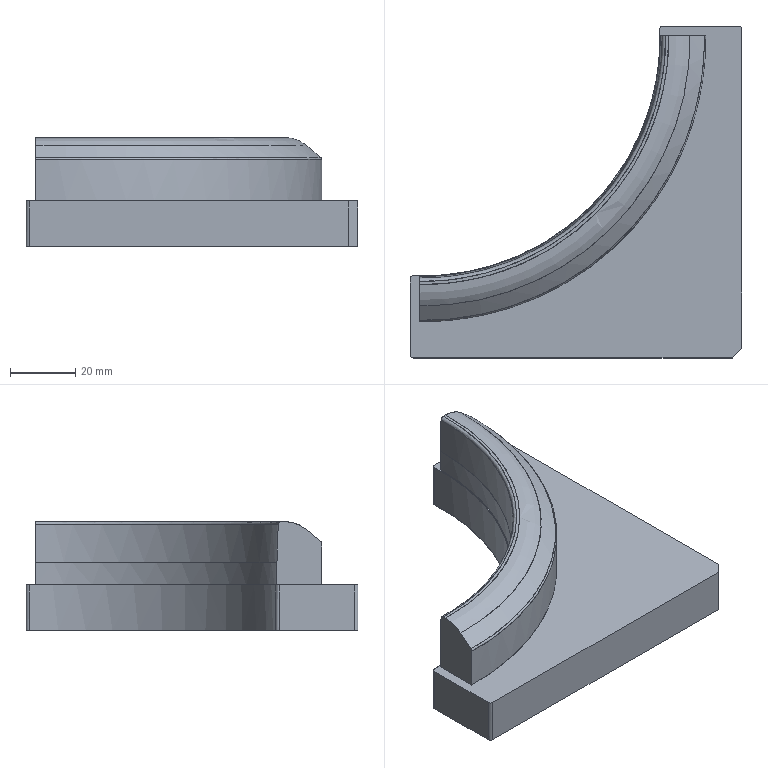NC program | PowerMill | posted with a generic post | part box 102 x 102 x 33.478 mm
Lines 27590 to 28295 of 321973:
N27687 M6
N27688 S18000 M03
N27689 G00 G90 X0.0 Y0.0
N27690 G43 Z10.798 H7
N27691
N27692 G05 P10000 R8
N27693 X17.1874 Y-14.3161
N27694 Z-7.9702
N27695 G01 Z-9.1702 F1200.0
N27696 Z-9.0886 F2000.0
N27697 X17.1872 Y-14.3163 Z-9.0864
N27698 X17.1843 Y-14.3192 Z-9.0682
N27699 X17.1792 Y-14.3243 Z-9.0512
N27700 X17.1716 Y-14.3319 Z-9.0349
N27701 X17.1609 Y-14.3426 Z-9.0187
N27702 X17.1455 Y-14.358 Z-9.0005
N27703 X17.1251 Y-14.3784 Z-8.9779
N27704 X17.1006 Y-14.4028 Z-8.9608
N27705 X17.0618 Y-14.4417 Z-8.9372
N27706 X17.0164 Y-14.4871 Z-8.9136
N27707 X16.9789 Y-14.5246 Z-8.8964
N27708 X16.9405 Y-14.563 Z-8.8811
N27709 X16.9017 Y-14.6018 Z-8.8675
N27710 X16.8627 Y-14.6408 Z-8.855
N27711 X16.8156 Y-14.6878 Z-8.841
N27712 X16.7764 Y-14.7271 Z-8.8301
N27713 X16.737 Y-14.7664 Z-8.82
N27714 X16.6975 Y-14.8059 Z-8.811
N27715 X16.6147 Y-14.8888 Z-8.7951
N27716 X16.5048 Y-14.9986 Z-8.7757
N27717 X16.3947 Y-15.1088 Z-8.7593
N27718 X16.2844 Y-15.2191 Z-8.7465
N27719 X16.1739 Y-15.3296 Z-8.7368
N27720 X16.0663 Y-15.4372 Z-8.7292
N27721 X15.9586 Y-15.5449 Z-8.7236
N27722 X15.8509 Y-15.6526 Z-8.7206
N27723 X15.7432 Y-15.7603 Z-8.7203
N27724 X15.6355 Y-15.868 Z-8.7216
N27725 X15.5787 Y-15.9248 Z-8.7227
N27726 X15.522 Y-15.9815 Z-8.7245
N27727 X15.4652 Y-16.0382 Z-8.7272
N27728 X15.4085 Y-16.0949 Z-8.7305
N27729 X15.3518 Y-16.1516 Z-8.7345
N27730 X15.2713 Y-16.2322 Z-8.7409
N27731 X15.2006 Y-16.3029 Z-8.7476
N27732 X15.1441 Y-16.3594 Z-8.7537
N27733 X15.0876 Y-16.4159 Z-8.7606
N27734 X15.0311 Y-16.4723 Z-8.7689
N27735 X14.975 Y-16.5285 Z-8.7791
N27736 X14.8879 Y-16.6156 Z-8.795
N27737 X14.8173 Y-16.6862 Z-8.8088
N27738 X14.7615 Y-16.742 Z-8.8224
N27739 X14.7057 Y-16.7978 Z-8.8378
N27740 X14.6663 Y-16.8372 Z-8.8482
N27741 X14.6274 Y-16.8761 Z-8.8578
N27742 X14.5955 Y-16.908 Z-8.8684
N27743 X14.554 Y-16.9494 Z-8.8851
N27744 X14.5371 Y-16.9664 Z-8.8917
N27745 X14.5202 Y-16.9833 Z-8.8987
N27746 X14.5024 Y-17.0011 Z-8.9068
N27747 X14.4775 Y-17.026 Z-8.9188
N27748 X14.4502 Y-17.0533 Z-8.9331
N27749 X14.4315 Y-17.072 Z-8.9439
N27750 X14.4155 Y-17.0879 Z-8.9542
N27751 X14.4071 Y-17.0964 Z-8.9607
N27752 X14.398 Y-17.1055 Z-8.9685
N27753 X14.3839 Y-17.1196 Z-8.9815
N27754 X14.3724 Y-17.1311 Z-8.9927
N27755 X14.365 Y-17.1385 Z-9.0003
N27756 X14.3605 Y-17.143 Z-9.0051
N27757 X14.3585 Y-17.145 Z-9.0077
N27758 X14.3532 Y-17.1503 Z-9.0163
N27759 X14.3369 Y-17.1666 Z-9.0403
N27760 X14.3258 Y-17.1777 Z-9.0585
N27761 X14.3186 Y-17.1849 Z-9.0746
N27762 X14.3169 Y-17.1866 Z-9.0798
N27763 X14.3162 Y-17.1872 Z-9.0854
N27764 Z-9.1727
N27765 X13.1725 Y-18.2603 Z-9.1688
N27766 Z-9.0851
N27767 X13.1761 Y-18.2567 Z-9.0569
N27768 X13.1783 Y-18.2544 Z-9.0391
N27769 X13.1824 Y-18.2503 Z-9.018
N27770 X13.1878 Y-18.2449 Z-9.0013
N27771 X13.1919 Y-18.2409 Z-8.9928
N27772 X13.2239 Y-18.2089 Z-8.9534
N27773 X13.2544 Y-18.1784 Z-8.9205
N27774 X13.2841 Y-18.1487 Z-8.8929
N27775 X13.3096 Y-18.1231 Z-8.8729
N27776 X13.3413 Y-18.0914 Z-8.8522
N27777 X13.3766 Y-18.0562 Z-8.8302
N27778 X13.4015 Y-18.0313 Z-8.8147
N27779 X13.427 Y-18.0057 Z-8.8012
N27780 X13.4913 Y-17.9414 Z-8.7708
N27781 X13.556 Y-17.8768 Z-8.7421
N27782 X13.6211 Y-17.8117 Z-8.7156
N27783 X13.6867 Y-17.746 Z-8.6916
N27784 X13.7529 Y-17.6799 Z-8.6703
N27785 X13.8194 Y-17.6134 Z-8.6512
N27786 X13.8861 Y-17.5466 Z-8.6337
N27787 X13.953 Y-17.4798 Z-8.6169
N27788 X14.0198 Y-17.413 Z-8.6005
N27789 X14.1145 Y-17.3182 Z-8.5798
N27790 X14.2281 Y-17.2046 Z-8.5585
N27791 X14.3901 Y-17.0426 Z-8.5314
N27792 X14.533 Y-16.8998 Z-8.51
N27793 X14.6562 Y-16.7766 Z-8.4948
N27794 X14.7763 Y-16.6564 Z-8.4825
N27795 X14.9314 Y-16.5014 Z-8.4679
N27796 X15.0866 Y-16.3462 Z-8.4564
N27797 X15.2418 Y-16.1909 Z-8.4483
N27798 X15.3711 Y-16.0617 Z-8.4425
N27799 X15.5044 Y-15.9284 Z-8.4387
N27800 X15.6861 Y-15.7466 Z-8.4368
N27801 X15.7937 Y-15.639 Z-8.4366
N27802 X15.9346 Y-15.4982 Z-8.4394
N27803 X16.005 Y-15.4277 Z-8.4406
N27804 X16.0585 Y-15.3743 Z-8.4422
N27805 X16.1119 Y-15.3209 Z-8.4444
N27806 X16.1653 Y-15.2675 Z-8.4469
N27807 X16.2272 Y-15.2056 Z-8.45
N27808 X16.2806 Y-15.1522 Z-8.4529
N27809 X16.334 Y-15.0988 Z-8.4559
N27810 X16.3874 Y-15.0454 Z-8.4595
N27811 X16.5443 Y-14.8885 Z-8.4716
N27812 X16.701 Y-14.7317 Z-8.4866
N27813 X16.8576 Y-14.5752 Z-8.5049
N27814 X17.0139 Y-14.4188 Z-8.5268
N27815 X17.1218 Y-14.3109 Z-8.5439
N27816 X17.2617 Y-14.1711 Z-8.569
N27817 X17.3907 Y-14.0421 Z-8.5957
N27818 X17.5114 Y-13.9214 Z-8.6243
N27819 X17.6252 Y-13.8075 Z-8.6551
N27820 X17.7334 Y-13.6994 Z-8.688
N27821 X17.7938 Y-13.6389 Z-8.7083
N27822 X17.8157 Y-13.617 Z-8.7163
N27823 X17.8375 Y-13.5952 Z-8.7249
N27824 X17.8623 Y-13.5705 Z-8.7351
N27825 X17.8935 Y-13.5392 Z-8.7486
N27826 X17.9366 Y-13.4961 Z-8.768
N27827 X17.9793 Y-13.4534 Z-8.7882
N27828 X18.0101 Y-13.4227 Z-8.8035
N27829 X18.0343 Y-13.3985 Z-8.8163
N27830 X18.0553 Y-13.3775 Z-8.828
N27831 X18.0759 Y-13.3568 Z-8.8408
N27832 X18.0961 Y-13.3366 Z-8.8553
N27833 X18.1178 Y-13.315 Z-8.8713
N27834 X18.1469 Y-13.2858 Z-8.8943
N27835 X18.1677 Y-13.2651 Z-8.9123
N27836 X18.1859 Y-13.2468 Z-8.9306
N27837 X18.2063 Y-13.2265 Z-8.9518
N27838 X18.2192 Y-13.2136 Z-8.9673
N27839 X18.2305 Y-13.2023 Z-8.985
N27840 X18.242 Y-13.1907 Z-9.0085
N27841 X18.2494 Y-13.1833 Z-9.0271
N27842 X18.253 Y-13.1798 Z-9.045
N27843 X18.258 Y-13.1747 Z-9.0668
N27844 X18.2602 Y-13.1726 Z-9.0827
N27845 Z-9.0832
N27846 Z-9.1693
N27847 X18.9879 Y-12.3742 Z-9.1709
N27848 Z-9.0831
N27849 X18.986 Y-12.3761 Z-9.0654
N27850 X18.9578 Y-12.4043 Z-8.9744
N27851 X18.9343 Y-12.4278 Z-8.9397
N27852 X18.9079 Y-12.4542 Z-8.9052
N27853 X18.8818 Y-12.4802 Z-8.8761
N27854 X18.8549 Y-12.5071 Z-8.8507
N27855 X18.8187 Y-12.5433 Z-8.8209
N27856 X18.7789 Y-12.5832 Z-8.7918
N27857 X18.7322 Y-12.6299 Z-8.7615
N27858 X18.6769 Y-12.6852 Z-8.7293
N27859 X18.6131 Y-12.7489 Z-8.6961
N27860 X18.5588 Y-12.8033 Z-8.6705
N27861 X18.5128 Y-12.8492 Z-8.6503
N27862 X18.4724 Y-12.8897 Z-8.6337
N27863 X18.4318 Y-12.9302 Z-8.6178
N27864 X18.3435 Y-13.0185 Z-8.5859
N27865 X18.2505 Y-13.1116 Z-8.5554
N27866 X18.157 Y-13.205 Z-8.5275
N27867 X18.056 Y-13.3061 Z-8.4999
N27868 X17.9333 Y-13.4288 Z-8.4693
N27869 X17.8061 Y-13.556 Z-8.4407
N27870 X17.7019 Y-13.6601 Z-8.4193
N27871 X17.6072 Y-13.7549 Z-8.4014
N27872 X17.5123 Y-13.8498 Z-8.385
N27873 X17.4173 Y-13.9447 Z-8.3701
N27874 X17.2755 Y-14.0866 Z-8.3489
N27875 X17.1335 Y-14.2285 Z-8.33
N27876 X16.9914 Y-14.3707 Z-8.314
N27877 X16.7971 Y-14.5649 Z-8.2948
N27878 X16.6028 Y-14.7593 Z-8.2788
N27879 X16.4083 Y-14.9538 Z-8.2663
N27880 X16.2137 Y-15.1484 Z-8.2567
N27881 X16.0151 Y-15.3469 Z-8.2503
N27882 X15.8203 Y-15.5418 Z-8.247
N27883 X15.6056 Y-15.7565 Z-8.2463
N27884 X15.3909 Y-15.9712 Z-8.2492
N27885 X15.1762 Y-16.1858 Z-8.2556
N27886 X14.9899 Y-16.3721 Z-8.2639
N27887 X14.7934 Y-16.5686 Z-8.2762
N27888 X14.6126 Y-16.7495 Z-8.2905
N27889 X14.4138 Y-16.9483 Z-8.3096
N27890 X14.2552 Y-17.1068 Z-8.3268
N27891 X14.0916 Y-17.2704 Z-8.348
N27892 X13.9134 Y-17.4487 Z-8.3749
N27893 X13.7526 Y-17.6095 Z-8.402
N27894 X13.61 Y-17.752 Z-8.4291
N27895 X13.4788 Y-17.8832 Z-8.4576
N27896 X13.3376 Y-18.0244 Z-8.4918
N27897 X13.2131 Y-18.149 Z-8.5253
N27898 X13.0997 Y-18.2623 Z-8.5593
N27899 X12.9978 Y-18.3643 Z-8.5934
N27900 X12.9046 Y-18.4575 Z-8.6282
N27901 X12.8207 Y-18.5413 Z-8.663
N27902 X12.7515 Y-18.6106 Z-8.695
N27903 X12.6913 Y-18.6708 Z-8.7262
N27904 X12.6373 Y-18.7247 Z-8.7578
N27905 X12.6092 Y-18.7529 Z-8.7759
N27906 X12.5812 Y-18.7809 Z-8.7944
N27907 X12.5534 Y-18.8086 Z-8.8137
N27908 X12.5265 Y-18.8356 Z-8.835
N27909 X12.5003 Y-18.8617 Z-8.8582
N27910 X12.4761 Y-18.886 Z-8.8812
N27911 X12.4489 Y-18.9132 Z-8.9106
N27912 X12.4256 Y-18.9364 Z-8.94
N27913 X12.4057 Y-18.9564 Z-8.9701
N27914 X12.3998 Y-18.9623 Z-8.9902
N27915 X12.3891 Y-18.973 Z-9.0198
N27916 X12.3808 Y-18.9813 Z-9.0449
N27917 X12.376 Y-18.986 Z-9.0656
N27918 X12.3741 Y-18.988 Z-9.0845
N27919 Z-9.1723
N27920 X11.7287 Y-19.5626 Z-9.1585
N27921 Z-9.0811
N27922 X11.7298 Y-19.5615 Z-9.0612
N27923 X11.732 Y-19.5594 Z-9.0411
N27924 X11.736 Y-19.5554 Z-9.0221
N27925 X11.7415 Y-19.5499 Z-9.0039
N27926 X11.7479 Y-19.5434 Z-8.9863
N27927 X11.7613 Y-19.53 Z-8.9561
N27928 X11.7776 Y-19.5138 Z-8.9268
N27929 X11.7969 Y-19.4944 Z-8.8983
N27930 X11.8195 Y-19.4718 Z-8.8705
N27931 X11.8458 Y-19.4456 Z-8.8433
N27932 X11.8749 Y-19.4164 Z-8.8152
N27933 X11.8956 Y-19.3957 Z-8.7955
N27934 X11.9172 Y-19.3741 Z-8.7779
N27935 X11.965 Y-19.3263 Z-8.7427
N27936 X12.0137 Y-19.2777 Z-8.71
N27937 X12.0631 Y-19.2282 Z-8.6798
N27938 X12.1134 Y-19.1779 Z-8.6522
N27939 X12.1709 Y-19.1204 Z-8.6235
N27940 X12.2222 Y-19.0692 Z-8.5994
N27941 X12.2735 Y-19.0178 Z-8.576
N27942 X12.345 Y-18.9463 Z-8.5461
N27943 X12.4304 Y-18.861 Z-8.5143
N27944 X12.5486 Y-18.7427 Z-8.4738
N27945 X12.6754 Y-18.616 Z-8.4343
N27946 X12.802 Y-18.4894 Z-8.3989
N27947 X12.9472 Y-18.3441 Z-8.3624
N27948 X13.1012 Y-18.1901 Z-8.3275
N27949 X13.2661 Y-18.0253 Z-8.2942
N27950 X13.4452 Y-17.8462 Z-8.2618
N27951 X13.6377 Y-17.6536 Z-8.2309
N27952 X13.8074 Y-17.4839 Z-8.2069
N27953 X13.9773 Y-17.314 Z-8.186
N27954 X14.1473 Y-17.144 Z-8.1675
N27955 X14.3175 Y-16.9739 Z-8.1512
N27956 X14.4906 Y-16.8008 Z-8.1366
N27957 X14.6638 Y-16.6276 Z-8.1244
N27958 X14.9151 Y-16.3763 Z-8.1107
N27959 X15.1634 Y-16.128 Z-8.1011
N27960 X15.4128 Y-15.8786 Z-8.0955
N27961 X15.6661 Y-15.6252 Z-8.0937
N27962 X15.8882 Y-15.4032 Z-8.0953
N27963 X16.1192 Y-15.1721 Z-8.1007
N27964 X16.2913 Y-15.0 Z-8.1067
N27965 X16.4771 Y-14.8143 Z-8.116
N27966 X16.6278 Y-14.6636 Z-8.1245
N27967 X16.7307 Y-14.5606 Z-8.1313
N27968 X16.8336 Y-14.4578 Z-8.139
N27969 X16.9365 Y-14.3549 Z-8.1474
N27970 X17.0393 Y-14.2521 Z-8.1569
N27971 X17.2621 Y-14.0292 Z-8.18
N27972 X17.4626 Y-13.8287 Z-8.2043
N27973 X17.651 Y-13.6403 Z-8.2306
N27974 X17.8466 Y-13.4448 Z-8.2617
N27975 X18.0287 Y-13.2626 Z-8.2941
N27976 X18.1664 Y-13.125 Z-8.3219
N27977 X18.3141 Y-12.9773 Z-8.3556
N27978 X18.4719 Y-12.8194 Z-8.3949
N27979 X18.5954 Y-12.696 Z-8.4283
N27980 X18.7018 Y-12.5895 Z-8.4604
N27981 X18.8055 Y-12.4858 Z-8.4947
N27982 X18.9038 Y-12.3876 Z-8.5298
N27983 X18.9882 Y-12.3032 Z-8.5633
N27984 X19.0637 Y-12.2277 Z-8.5968
N27985 X19.1081 Y-12.1832 Z-8.6183
N27986 X19.1525 Y-12.1388 Z-8.6402
N27987 X19.1968 Y-12.0946 Z-8.6628
N27988 X19.2406 Y-12.0507 Z-8.6869
N27989 X19.2838 Y-12.0076 Z-8.7132
N27990 X19.3259 Y-11.9654 Z-8.7425
N27991 X19.3672 Y-11.9241 Z-8.7742
N27992 X19.4079 Y-11.8835 Z-8.8075
N27993 X19.4426 Y-11.8487 Z-8.8369
N27994 X19.4569 Y-11.8344 Z-8.8512
N27995 X19.4725 Y-11.8188 Z-8.8712
N27996 X19.4899 Y-11.8015 Z-8.8953
N27997 X19.5125 Y-11.7788 Z-8.9257
N27998 X19.5278 Y-11.7635 Z-8.9488
N27999 X19.539 Y-11.7524 Z-8.9701
N28000 X19.5472 Y-11.7442 Z-8.9912
N28001 X19.553 Y-11.7384 Z-9.0131
N28002 X19.5563 Y-11.735 Z-9.0324
N28003 X19.5609 Y-11.7304 Z-9.064
N28004 X19.5627 Y-11.7286 Z-9.0828
N28005 Z-9.1508
N28006 X20.0604 Y-11.1602 Z-9.1594
N28007 Z-9.0869
N28008 X20.0573 Y-11.1633 Z-9.0553
N28009 X20.0515 Y-11.1691 Z-9.0242
N28010 X20.0429 Y-11.1777 Z-8.9933
N28011 X20.0315 Y-11.1892 Z-8.9626
N28012 X20.0169 Y-11.2037 Z-8.932
N28013 X19.9991 Y-11.2215 Z-8.9014
N28014 X19.9778 Y-11.2428 Z-8.8709
N28015 X19.9528 Y-11.2679 Z-8.8404
N28016 X19.9267 Y-11.2939 Z-8.8125
N28017 X19.8929 Y-11.3278 Z-8.78
N28018 X19.8546 Y-11.366 Z-8.7471
N28019 X19.8116 Y-11.4091 Z-8.7137
N28020 X19.7631 Y-11.4576 Z-8.6796
N28021 X19.7081 Y-11.5125 Z-8.6446
N28022 X19.6454 Y-11.5753 Z-8.6083
N28023 X19.5731 Y-11.6476 Z-8.5703
N28024 X19.4913 Y-11.7293 Z-8.5314
N28025 X19.4186 Y-11.8021 Z-8.4997
N28026 X19.3555 Y-11.8652 Z-8.4741
N28027 X19.3003 Y-11.9203 Z-8.4529
N28028 X19.2578 Y-11.9628 Z-8.4374
N28029 X19.1546 Y-12.066 Z-8.401
N28030 X19.0509 Y-12.1697 Z-8.3675
N28031 X18.9468 Y-12.2738 Z-8.3371
N28032 X18.8424 Y-12.3783 Z-8.3088
N28033 X18.6919 Y-12.5288 Z-8.2703
N28034 X18.5552 Y-12.6655 Z-8.2387
N28035 X18.3866 Y-12.834 Z-8.2036
N28036 X18.2057 Y-13.0149 Z-8.1698
N28037 X18.0083 Y-13.2124 Z-8.1368
N28038 X17.8379 Y-13.3828 Z-8.1109
N28039 X17.6353 Y-13.5854 Z-8.0832
N28040 X17.446 Y-13.7747 Z-8.0609
N28041 X17.2589 Y-13.9617 Z-8.0417
N28042 X17.0633 Y-14.1573 Z-8.0234
N28043 X16.8934 Y-14.3273 Z-8.0104
N28044 X16.7195 Y-14.5011 Z-7.9984
N28045 X16.5456 Y-14.675 Z-7.9879
N28046 X16.3717 Y-14.8489 Z-7.9801
N28047 X16.1977 Y-15.0229 Z-7.974
N28048 X15.9804 Y-15.2402 Z-7.9676
N28049 X15.7631 Y-15.4575 Z-7.9649
N28050 X15.6208 Y-15.5998 Z-7.964
N28051 X15.4785 Y-15.7422 Z-7.9647
N28052 X15.3362 Y-15.8845 Z-7.9662
N28053 X15.1939 Y-16.0268 Z-7.9686
N28054 X15.0516 Y-16.1691 Z-7.9725
N28055 X14.8377 Y-16.3829 Z-7.9808
N28056 X14.624 Y-16.5967 Z-7.9913
N28057 X14.4102 Y-16.8104 Z-8.0042
N28058 X14.2394 Y-16.9813 Z-8.0169
N28059 X14.0685 Y-17.1521 Z-8.0315
N28060 X13.8978 Y-17.3228 Z-8.0478
N28061 X13.7053 Y-17.5153 Z-8.0687
N28062 X13.513 Y-17.7076 Z-8.0926
N28063 X13.321 Y-17.8997 Z-8.1199
N28064 X13.1693 Y-18.0513 Z-8.1437
N28065 X13.0178 Y-18.2029 Z-8.1693
N28066 X12.8664 Y-18.3542 Z-8.1971
N28067 X12.7154 Y-18.5052 Z-8.2279
N28068 X12.5648 Y-18.6559 Z-8.2621
N28069 X12.4623 Y-18.7583 Z-8.2874
N28070 X12.36 Y-18.8606 Z-8.3136
N28071 X12.2579 Y-18.9627 Z-8.3413
N28072 X12.1562 Y-19.0644 Z-8.3717
N28073 X12.055 Y-19.1657 Z-8.4051
N28074 X11.9405 Y-19.2802 Z-8.4461
N28075 X11.8319 Y-19.3887 Z-8.4881
N28076 X11.7408 Y-19.4798 Z-8.5265
N28077 X11.6633 Y-19.5573 Z-8.5625
N28078 X11.5944 Y-19.6263 Z-8.598
N28079 X11.5302 Y-19.6904 Z-8.6348
N28080 X11.4656 Y-19.7551 Z-8.6747
N28081 X11.4131 Y-19.8075 Z-8.7102
N28082 X11.3679 Y-19.8527 Z-8.7445
N28083 X11.3279 Y-19.8928 Z-8.7787
N28084 X11.2918 Y-19.9289 Z-8.8138
N28085 X11.2697 Y-19.9509 Z-8.838
N28086 X11.2446 Y-19.9761 Z-8.8696
N28087 X11.223 Y-19.9977 Z-8.9016
N28088 X11.2047 Y-20.0159 Z-8.9338
N28089 X11.1896 Y-20.0311 Z-8.9664
N28090 X11.1774 Y-20.0433 Z-8.9993
N28091 X11.168 Y-20.0526 Z-9.0327
N28092 X11.1627 Y-20.0579 Z-9.059
N28093 X11.1604 Y-20.0602 Z-9.0808
N28094 Z-9.1798
N28095 X10.6533 Y-20.4966 Z-9.1585
N28096 Z-9.0817
N28097 X10.656 Y-20.494 Z-9.0477
N28098 X10.6598 Y-20.4902 Z-9.0221
N28099 X10.6654 Y-20.4846 Z-8.9999
N28100 X10.6749 Y-20.475 Z-8.972
N28101 X10.688 Y-20.4619 Z-8.9409
N28102 X10.7056 Y-20.4443 Z-8.9058
N28103 X10.7239 Y-20.4261 Z-8.8751
N28104 X10.7403 Y-20.4097 Z-8.8515
N28105 X10.7568 Y-20.3931 Z-8.831
N28106 X10.7929 Y-20.357 Z-8.7902
N28107 X10.8306 Y-20.3193 Z-8.7526
N28108 X10.871 Y-20.279 Z-8.7168
N28109 X10.9155 Y-20.2344 Z-8.6816
N28110 X10.966 Y-20.184 Z-8.6461
N28111 X11.0257 Y-20.1243 Z-8.608
N28112 X11.0988 Y-20.0511 Z-8.565
N28113 X11.1759 Y-19.9741 Z-8.5239
N28114 X11.2597 Y-19.8902 Z-8.4833
N28115 X11.3527 Y-19.7973 Z-8.4423
N28116 X11.4589 Y-19.691 Z-8.3994
N28117 X11.5738 Y-19.5761 Z-8.3569
N28118 X11.697 Y-19.4529 Z-8.3154
N28119 X11.8312 Y-19.3188 Z-8.2741
N28120 X11.9806 Y-19.1694 Z-8.2319
N28121 X12.0944 Y-19.0555 Z-8.2025
N28122 X12.2136 Y-18.9364 Z-8.1741
N28123 X12.3329 Y-18.817 Z-8.1476
N28124 X12.4525 Y-18.6975 Z-8.1224
N28125 X12.5721 Y-18.5778 Z-8.0987
N28126 X12.692 Y-18.458 Z-8.0767
N28127 X12.8119 Y-18.338 Z-8.0565
N28128 X12.9845 Y-18.1654 Z-8.0286
N28129 X13.1573 Y-17.9926 Z-8.0035
N28130 X13.3439 Y-17.806 Z-7.9796
N28131 X13.5018 Y-17.6482 Z-7.9607
N28132 X13.6597 Y-17.4903 Z-7.9435
N28133 X13.8177 Y-17.3323 Z-7.9282
N28134 X13.9757 Y-17.1742 Z-7.9143
N28135 X14.1339 Y-17.0161 Z-7.9021
N28136 X14.3342 Y-16.8157 Z-7.8881
N28137 X14.5346 Y-16.6153 Z-7.8767
N28138 X14.7633 Y-16.3866 Z-7.866
N28139 X14.9663 Y-16.1836 Z-7.8592
N28140 X15.2048 Y-15.9452 Z-7.8531
N28141 X15.4432 Y-15.7067 Z-7.8505
N28142 X15.6571 Y-15.4928 Z-7.85
N28143 X15.8889 Y-15.2611 Z-7.8524
N28144 X16.1784 Y-14.9716 Z-7.8588
N28145 X16.3701 Y-14.7799 Z-7.8652
N28146 X16.5617 Y-14.5882 Z-7.8733
N28147 X16.7533 Y-14.3966 Z-7.884
N28148 X16.9448 Y-14.2051 Z-7.897
N28149 X17.1236 Y-14.0263 Z-7.9102
N28150 X17.3024 Y-13.8476 Z-7.9254
N28151 X17.481 Y-13.6689 Z-7.9426
N28152 X17.6595 Y-13.4904 Z-7.9619
N28153 X17.7739 Y-13.376 Z-7.9757
N28154 X17.8883 Y-13.2617 Z-7.9897
N28155 X18.0025 Y-13.1474 Z-8.0048
N28156 X18.1167 Y-13.0332 Z-8.0215
N28157 X18.2858 Y-12.8641 Z-8.0478
N28158 X18.4548 Y-12.6952 Z-8.0763
N28159 X18.6235 Y-12.5265 Z-8.1075
N28160 X18.7918 Y-12.3581 Z-8.142
N28161 X18.9598 Y-12.1901 Z-8.1799
N28162 X19.0913 Y-12.0586 Z-8.212
N28163 X19.1738 Y-11.9761 Z-8.2334
N28164 X19.2614 Y-11.8885 Z-8.2574
N28165 X19.3609 Y-11.7891 Z-8.2865
N28166 X19.475 Y-11.6749 Z-8.3224
N28167 X19.5965 Y-11.5535 Z-8.364
N28168 X19.7029 Y-11.4471 Z-8.4039
N28169 X19.796 Y-11.3539 Z-8.4418
N28170 X19.8787 Y-11.2712 Z-8.4782
N28171 X19.958 Y-11.192 Z-8.5161
N28172 X20.0365 Y-11.1134 Z-8.5572
N28173 X20.1002 Y-11.0497 Z-8.5933
N28174 X20.1624 Y-10.9876 Z-8.6316
N28175 X20.2166 Y-10.9333 Z-8.6686
N28176 X20.2651 Y-10.8848 Z-8.7056
N28177 X20.3091 Y-10.8409 Z-8.7432
N28178 X20.3491 Y-10.8008 Z-8.7817
N28179 X20.3859 Y-10.764 Z-8.8216
N28180 X20.4011 Y-10.7489 Z-8.84
N28181 X20.4188 Y-10.7311 Z-8.8642
N28182 X20.439 Y-10.711 Z-8.8955
N28183 X20.4572 Y-10.6927 Z-8.9287
N28184 X20.4712 Y-10.6788 Z-8.9592
N28185 X20.4813 Y-10.6686 Z-8.987
N28186 X20.4881 Y-10.6618 Z-9.0125
N28187 X20.4916 Y-10.6583 Z-9.0337
N28188 X20.4957 Y-10.6543 Z-9.0635
N28189 X20.4972 Y-10.6528 Z-9.0817
N28190 Z-9.17
N28191 X20.8916 Y-10.1877 Z-9.1653
N28192 X20.8915 Z-9.0805
N28193 X20.8906 Y-10.1887 Z-9.0681
N28194 X20.8877 Y-10.1916 Z-9.0418
N28195 X20.8826 Y-10.1966 Z-9.0162
N28196 X20.876 Y-10.2032 Z-8.9913
N28197 X20.8686 Y-10.2106 Z-8.967
N28198 X20.8562 Y-10.223 Z-8.9345
N28199 X20.8405 Y-10.2387 Z-8.9017
N28200 X20.8214 Y-10.2578 Z-8.8685
N28201 X20.7986 Y-10.2806 Z-8.8347
N28202 X20.7717 Y-10.3075 Z-8.8001
N28203 X20.7401 Y-10.3391 Z-8.7645
N28204 X20.7031 Y-10.3761 Z-8.7275
N28205 X20.6601 Y-10.4191 Z-8.6892
N28206 X20.6153 Y-10.464 Z-8.6529
N28207 X20.5753 Y-10.5039 Z-8.6232
N28208 X20.5228 Y-10.5564 Z-8.5875
N28209 X20.4695 Y-10.6097 Z-8.5544
N28210 X20.4116 Y-10.6676 Z-8.5211
N28211 X20.3445 Y-10.7347 Z-8.4853
N28212 X20.2645 Y-10.8147 Z-8.4458
N28213 X20.1675 Y-10.9117 Z-8.4017
N28214 X20.0861 Y-10.9932 Z-8.3673
N28215 X20.0174 Y-11.0618 Z-8.3401
N28216 X19.9581 Y-11.1211 Z-8.3176
N28217 X19.9015 Y-11.1777 Z-8.2973
N28218 X19.8448 Y-11.2344 Z-8.2778
N28219 X19.7144 Y-11.3648 Z-8.2358
N28220 X19.5836 Y-11.4956 Z-8.1968
N28221 X19.4524 Y-11.6268 Z-8.1604
N28222 X19.3209 Y-11.7583 Z-8.1264
N28223 X19.1891 Y-11.8902 Z-8.0947
N28224 X19.0569 Y-12.0223 Z-8.0655
N28225 X18.897 Y-12.1822 Z-8.0328
N28226 X18.7208 Y-12.3584 Z-7.9994
N28227 X18.5443 Y-12.5349 Z-7.9692
N28228 X18.3363 Y-12.7429 Z-7.9365
N28229 X18.1279 Y-12.9513 Z-7.9069
N28230 X17.9194 Y-13.1598 Z-7.8806
N28231 X17.7107 Y-13.3685 Z-7.8572
N28232 X17.5018 Y-13.5774 Z-7.836
N28233 X17.2802 Y-13.799 Z-7.8164
N28234 X17.0585 Y-14.0207 Z-7.7994
N28235 X16.789 Y-14.2902 Z-7.7823
N28236 X16.5191 Y-14.5601 Z-7.7687
N28237 X16.2304 Y-14.8488 Z-7.7577
N28238 X15.9397 Y-15.1396 Z-7.7506
N28239 X15.6584 Y-15.4208 Z-7.7473
N28240 X15.3742 Y-15.705 Z-7.7477
N28241 X15.0748 Y-16.0044 Z-7.7519
N28242 X14.8605 Y-16.2187 Z-7.7573
N28243 X14.6463 Y-16.433 Z-7.7649
N28244 X14.4321 Y-16.6471 Z-7.7746
N28245 X14.2505 Y-16.8287 Z-7.7849
N28246 X14.0689 Y-17.0103 Z-7.7962
N28247 X13.8874 Y-17.1919 Z-7.8087
N28248 X13.7059 Y-17.3733 Z-7.8238
N28249 X13.5246 Y-17.5546 Z-7.8409
N28250 X13.3078 Y-17.7714 Z-7.8635
N28251 X13.0553 Y-18.024 Z-7.8936
N28252 X12.8233 Y-18.2559 Z-7.9248
N28253 X12.5857 Y-18.4935 Z-7.9607
N28254 X12.417 Y-18.6622 Z-7.9885
N28255 X12.2486 Y-18.8306 Z-8.0195
N28256 X12.0804 Y-18.9988 Z-8.0533
N28257 X11.9695 Y-19.1098 Z-8.077
N28258 X11.8586 Y-19.2206 Z-8.1022
N28259 X11.748 Y-19.3312 Z-8.129
N28260 X11.6232 Y-19.456 Z-8.1613
N28261 X11.4735 Y-19.6057 Z-8.2031
N28262 X11.3441 Y-19.7351 Z-8.2422
N28263 X11.2347 Y-19.8445 Z-8.2779
N28264 X11.1258 Y-19.9534 Z-8.3161
N28265 X11.0175 Y-20.0617 Z-8.3572
N28266 X10.9532 Y-20.126 Z-8.3835
N28267 X10.8892 Y-20.19 Z-8.4112
N28268 X10.8255 Y-20.2537 Z-8.4403
N28269 X10.7526 Y-20.3266 Z-8.4759
N28270 X10.6899 Y-20.3894 Z-8.5088
N28271 X10.6278 Y-20.4514 Z-8.5443
N28272 X10.5736 Y-20.5056 Z-8.5779
N28273 X10.5129 Y-20.5663 Z-8.6182
N28274 X10.4587 Y-20.6205 Z-8.6579
N28275 X10.4109 Y-20.6683 Z-8.6967
N28276 X10.3687 Y-20.7105 Z-8.7349
N28277 X10.3312 Y-20.748 Z-8.773
N28278 X10.298 Y-20.7812 Z-8.8111
N28279 X10.2686 Y-20.8106 Z-8.8494
N28280 X10.2551 Y-20.8241 Z-8.8693
N28281 X10.2411 Y-20.8381 Z-8.8939
N28282 X10.2264 Y-20.8528 Z-8.9247
N28283 X10.2121 Y-20.8671 Z-8.9611
N28284 X10.2012 Y-20.878 Z-8.9963
N28285 X10.1937 Y-20.8855 Z-9.0287
N28286 X10.1892 Y-20.89 Z-9.0578
N28287 X10.1876 Y-20.8917 Z-9.084
N28288 Z-9.1644
N28289 X9.7532 Y-21.2553 Z-9.1557
N28290 Z-9.0787
N28291 X9.7555 Y-21.253 Z-9.0525
N28292 X9.7608 Y-21.2477 Z-9.0233
N28293 X9.7695 Y-21.239 Z-8.9886
N28294 X9.7812 Y-21.2273 Z-8.9511
N28295 X9.7955 Y-21.213 Z-8.9147
N28296 X9.8126 Y-21.1959 Z-8.8795
N28297 X9.8325 Y-21.176 Z-8.8454
N28298 X9.8553 Y-21.1532 Z-8.8125
N28299 X9.881 Y-21.1275 Z-8.7809
N28300 X9.9177 Y-21.0908 Z-8.7407
N28301 X9.9596 Y-21.0489 Z-8.6996
N28302 X10.0074 Y-21.0011 Z-8.6572
N28303 X10.0601 Y-20.9484 Z-8.6149
N28304 X10.1091 Y-20.8994 Z-8.5791
N28305 X10.1527 Y-20.8558 Z-8.5496
N28306 X10.1951 Y-20.8134 Z-8.5229
N28307 X10.2704 Y-20.7381 Z-8.4792
N28308 X10.3465 Y-20.662 Z-8.4385
N28309 X10.4302 Y-20.5783 Z-8.3972
N28310 X10.5245 Y-20.484 Z-8.3543
N28311 X10.6312 Y-20.3773 Z-8.3096
N28312 X10.7434 Y-20.2651 Z-8.2663
N28313 X10.8434 Y-20.1651 Z-8.2305
N28314 X10.9316 Y-20.0769 Z-8.2008
N28315 X11.0111 Y-19.9974 Z-8.1755
N28316 X11.1452 Y-19.8633 Z-8.1356
N28317 X11.2798 Y-19.7287 Z-8.0985
N28318 X11.43 Y-19.5785 Z-8.06
N28319 X11.5652 Y-19.4433 Z-8.0277
N28320 X11.7006 Y-19.3079 Z-7.9974
N28321 X11.8362 Y-19.1723 Z-7.9691
N28322 X12.0179 Y-18.9906 Z-7.9337
N28323 X12.1999 Y-18.8086 Z-7.9016
N28324 X12.3822 Y-18.6263 Z-7.8722
N28325 X12.6226 Y-18.3859 Z-7.8368
N28326 X12.8702 Y-18.1383 Z-7.8044
N28327 X13.1256 Y-17.8829 Z-7.7749
N28328 X13.3637 Y-17.6448 Z-7.7508
N28329 X13.6321 Y-17.3764 Z-7.7271
N28330 X13.9006 Y-17.1079 Z-7.707
N28331 X14.1692 Y-16.8393 Z-7.6905
N28332 X14.4379 Y-16.5706 Z-7.677
N28333 X14.7067 Y-16.3018 Z-7.6665
N28334 X14.9978 Y-16.0107 Z-7.6588
N28335 X15.311 Y-15.6975 Z-7.6544
N28336 X15.6103 Y-15.3982 Z-7.6538
N28337 X15.9095 Y-15.099 Z-7.6568
N28338 X16.2087 Y-14.7998 Z-7.6637
N28339 X16.5079 Y-14.5006 Z-7.6744
N28340 X16.793 Y-14.2155 Z-7.688
N28341 X17.0781 Y-13.9304 Z-7.7051
N28342 X17.363 Y-13.6455 Z-7.726
N28343 X17.6363 Y-13.3722 Z-7.7495
N28344 X17.7199 Y-13.2886 Z-7.7579
N28345 X17.8034 Y-13.2051 Z-7.7667
N28346 X17.8869 Y-13.1216 Z-7.7757
N28347 X17.9705 Y-13.0381 Z-7.7849
N28348 X18.054 Y-12.9545 Z-7.7942
N28349 X18.1374 Y-12.8711 Z-7.8039
N28350 X18.2209 Y-12.7876 Z-7.8146
N28351 X18.4164 Y-12.5921 Z-7.8412
N28352 X18.6117 Y-12.3968 Z-7.87
N28353 X18.8068 Y-12.2017 Z-7.9012
N28354 X19.0017 Y-12.0068 Z-7.9359
N28355 X19.2073 Y-11.8012 Z-7.9762
N28356 X19.3835 Y-11.625 Z-8.0139
N28357 X19.562 Y-11.4465 Z-8.056
N28358 X19.7294 Y-11.2791 Z-8.0988
N28359 X19.8837 Y-11.1248 Z-8.1416
N28360 X20.026 Y-10.9825 Z-8.1846
N28361 X20.1583 Y-10.8502 Z-8.2282
N28362 X20.2824 Y-10.7261 Z-8.2729
N28363 X20.4011 Y-10.6074 Z-8.3194
N28364 X20.5028 Y-10.5057 Z-8.3625
N28365 X20.5987 Y-10.4098 Z-8.4069
N28366 X20.6895 Y-10.319 Z-8.4528
N28367 X20.7519 Y-10.2566 Z-8.4868
N28368 X20.8233 Y-10.1852 Z-8.5288
N28369 X20.8863 Y-10.1222 Z-8.5694
N28370 X20.943 Y-10.0655 Z-8.6098
N28371 X20.9946 Y-10.0139 Z-8.6507
N28372 X21.0421 Y-9.9664 Z-8.6924
N28373 X21.0858 Y-9.9227 Z-8.7353
N28374 X21.1264 Y-9.8821 Z-8.7795
N28375 X21.1536 Y-9.8549 Z-8.8131
N28376 X21.177 Y-9.8315 Z-8.8467
N28377 X21.1971 Y-9.8114 Z-8.8805
N28378 X21.2139 Y-9.7946 Z-8.9148
N28379 X21.2278 Y-9.7807 Z-8.9495
N28380 X21.2389 Y-9.7696 Z-8.9849
N28381 X21.2473 Y-9.7612 Z-9.021
N28382 X21.253 Y-9.7555 Z-9.0579
N28383 X21.2552 Y-9.7533 Z-9.0794
N28384 Z-9.1533
N28385 X21.5913 Y-9.3465 Z-9.172
N28386 Z-9.0729
N28387 X21.5906 Y-9.3472 Z-9.063
N28388 X21.5881 Y-9.3497 Z-9.0369
N28389 X21.5843 Y-9.3535 Z-9.0111
N28390 X21.5786 Y-9.3592 Z-8.986
N28391 X21.5707 Y-9.3671 Z-8.9605
N28392 X21.5619 Y-9.3759 Z-8.937